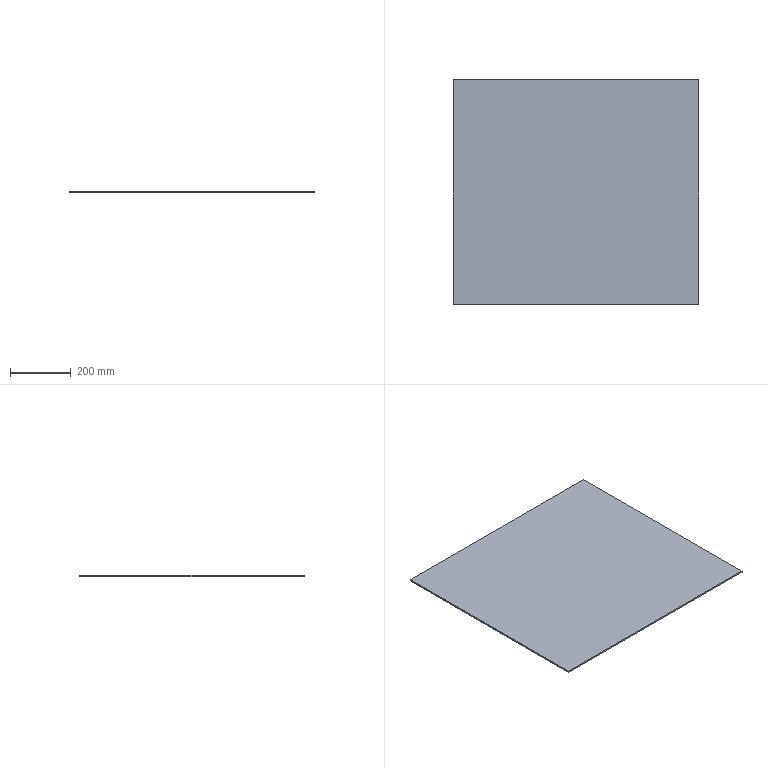Part | STEP file | Guide wheel mechanism revised.sldasm-Part-23 | 1 solid | 6 faces | box 810 x 740 x 5 mm | volume 2997000 mm3 | plane 6
STEP:
#1=CARTESIAN_POINT('',(-405.,740.,-505.));
#2=VERTEX_POINT('',#1);
#3=CARTESIAN_POINT('',(-405.,0.,-505.));
#4=VERTEX_POINT('',#3);
#5=CARTESIAN_POINT('',(-405.,740.,-505.));
#6=DIRECTION('',(0.,-1.,0.));
#7=VECTOR('',#6,1000.);
#8=LINE('',#5,#7);
#9=EDGE_CURVE('',#2,#4,#8,.T.);
#10=ORIENTED_EDGE('',*,*,#9,.F.);
#11=CARTESIAN_POINT('',(-405.,740.,-510.));
#12=VERTEX_POINT('',#11);
#13=CARTESIAN_POINT('',(-405.,740.,-510.));
#14=DIRECTION('',(0.,0.,1.));
#15=VECTOR('',#14,1000.);
#16=LINE('',#13,#15);
#17=EDGE_CURVE('',#12,#2,#16,.T.);
#18=ORIENTED_EDGE('',*,*,#17,.F.);
#19=CARTESIAN_POINT('',(-405.,0.,-510.));
#20=VERTEX_POINT('',#19);
#21=CARTESIAN_POINT('',(-405.,740.,-510.));
#22=DIRECTION('',(0.,-1.,0.));
#23=VECTOR('',#22,1000.);
#24=LINE('',#21,#23);
#25=EDGE_CURVE('',#12,#20,#24,.T.);
#26=ORIENTED_EDGE('',*,*,#25,.T.);
#27=CARTESIAN_POINT('',(-405.,0.,-510.));
#28=DIRECTION('',(0.,0.,1.));
#29=VECTOR('',#28,1000.);
#30=LINE('',#27,#29);
#31=EDGE_CURVE('',#20,#4,#30,.T.);
#32=ORIENTED_EDGE('',*,*,#31,.T.);
#33=EDGE_LOOP('',(#10,#18,#26,#32));
#34=FACE_OUTER_BOUND('',#33,.T.);
#35=CARTESIAN_POINT('',(-405.,740.,-510.));
#36=DIRECTION('',(-1.,0.,0.));
#37=DIRECTION('',(0.,-1.,0.));
#38=AXIS2_PLACEMENT_3D('',#35,#36,#37);
#39=PLANE('',#38);
#40=ADVANCED_FACE('',(#34),#39,.T.);
#41=CARTESIAN_POINT('',(405.,740.,-505.));
#42=VERTEX_POINT('',#41);
#43=CARTESIAN_POINT('',(-405.,740.,-505.));
#44=DIRECTION('',(-1.,0.,0.));
#45=VECTOR('',#44,1000.);
#46=LINE('',#43,#45);
#47=EDGE_CURVE('',#42,#2,#46,.T.);
#48=ORIENTED_EDGE('',*,*,#47,.F.);
#49=CARTESIAN_POINT('',(405.,740.,-510.));
#50=VERTEX_POINT('',#49);
#51=CARTESIAN_POINT('',(405.,740.,-510.));
#52=DIRECTION('',(0.,0.,1.));
#53=VECTOR('',#52,1000.);
#54=LINE('',#51,#53);
#55=EDGE_CURVE('',#50,#42,#54,.T.);
#56=ORIENTED_EDGE('',*,*,#55,.F.);
#57=CARTESIAN_POINT('',(-405.,740.,-510.));
#58=DIRECTION('',(-1.,0.,0.));
#59=VECTOR('',#58,1000.);
#60=LINE('',#57,#59);
#61=EDGE_CURVE('',#50,#12,#60,.T.);
#62=ORIENTED_EDGE('',*,*,#61,.T.);
#63=ORIENTED_EDGE('',*,*,#17,.T.);
#64=EDGE_LOOP('',(#48,#56,#62,#63));
#65=FACE_OUTER_BOUND('',#64,.T.);
#66=CARTESIAN_POINT('',(-405.,740.,-510.));
#67=DIRECTION('',(0.,1.,0.));
#68=DIRECTION('',(0.,0.,1.));
#69=AXIS2_PLACEMENT_3D('',#66,#67,#68);
#70=PLANE('',#69);
#71=ADVANCED_FACE('',(#65),#70,.T.);
#72=CARTESIAN_POINT('',(405.,0.,-505.));
#73=VERTEX_POINT('',#72);
#74=CARTESIAN_POINT('',(405.,740.,-505.));
#75=DIRECTION('',(0.,1.,0.));
#76=VECTOR('',#75,1000.);
#77=LINE('',#74,#76);
#78=EDGE_CURVE('',#73,#42,#77,.T.);
#79=ORIENTED_EDGE('',*,*,#78,.F.);
#80=CARTESIAN_POINT('',(405.,0.,-510.));
#81=VERTEX_POINT('',#80);
#82=CARTESIAN_POINT('',(405.,0.,-510.));
#83=DIRECTION('',(0.,0.,1.));
#84=VECTOR('',#83,1000.);
#85=LINE('',#82,#84);
#86=EDGE_CURVE('',#81,#73,#85,.T.);
#87=ORIENTED_EDGE('',*,*,#86,.F.);
#88=CARTESIAN_POINT('',(405.,740.,-510.));
#89=DIRECTION('',(0.,1.,0.));
#90=VECTOR('',#89,1000.);
#91=LINE('',#88,#90);
#92=EDGE_CURVE('',#81,#50,#91,.T.);
#93=ORIENTED_EDGE('',*,*,#92,.T.);
#94=ORIENTED_EDGE('',*,*,#55,.T.);
#95=EDGE_LOOP('',(#79,#87,#93,#94));
#96=FACE_OUTER_BOUND('',#95,.T.);
#97=CARTESIAN_POINT('',(405.,740.,-510.));
#98=DIRECTION('',(1.,0.,0.));
#99=DIRECTION('',(0.,1.,0.));
#100=AXIS2_PLACEMENT_3D('',#97,#98,#99);
#101=PLANE('',#100);
#102=ADVANCED_FACE('',(#96),#101,.T.);
#103=CARTESIAN_POINT('',(-405.,0.,-505.));
#104=DIRECTION('',(1.,0.,0.));
#105=VECTOR('',#104,1000.);
#106=LINE('',#103,#105);
#107=EDGE_CURVE('',#4,#73,#106,.T.);
#108=ORIENTED_EDGE('',*,*,#107,.F.);
#109=ORIENTED_EDGE('',*,*,#31,.F.);
#110=CARTESIAN_POINT('',(-405.,0.,-510.));
#111=DIRECTION('',(1.,0.,0.));
#112=VECTOR('',#111,1000.);
#113=LINE('',#110,#112);
#114=EDGE_CURVE('',#20,#81,#113,.T.);
#115=ORIENTED_EDGE('',*,*,#114,.T.);
#116=ORIENTED_EDGE('',*,*,#86,.T.);
#117=EDGE_LOOP('',(#108,#109,#115,#116));
#118=FACE_OUTER_BOUND('',#117,.T.);
#119=CARTESIAN_POINT('',(-405.,0.,-510.));
#120=DIRECTION('',(0.,-1.,0.));
#121=DIRECTION('',(0.,0.,-1.));
#122=AXIS2_PLACEMENT_3D('',#119,#120,#121);
#123=PLANE('',#122);
#124=ADVANCED_FACE('',(#118),#123,.T.);
#125=ORIENTED_EDGE('',*,*,#25,.F.);
#126=ORIENTED_EDGE('',*,*,#61,.F.);
#127=ORIENTED_EDGE('',*,*,#92,.F.);
#128=ORIENTED_EDGE('',*,*,#114,.F.);
#129=EDGE_LOOP('',(#125,#126,#127,#128));
#130=FACE_OUTER_BOUND('',#129,.T.);
#131=CARTESIAN_POINT('',(0.,0.,-510.));
#132=DIRECTION('',(0.,0.,1.));
#133=DIRECTION('',(1.,0.,0.));
#134=AXIS2_PLACEMENT_3D('',#131,#132,#133);
#135=PLANE('',#134);
#136=ADVANCED_FACE('',(#130),#135,.F.);
#137=ORIENTED_EDGE('',*,*,#9,.T.);
#138=ORIENTED_EDGE('',*,*,#107,.T.);
#139=ORIENTED_EDGE('',*,*,#78,.T.);
#140=ORIENTED_EDGE('',*,*,#47,.T.);
#141=EDGE_LOOP('',(#137,#138,#139,#140));
#142=FACE_OUTER_BOUND('',#141,.T.);
#143=CARTESIAN_POINT('',(0.,0.,-505.));
#144=DIRECTION('',(0.,0.,1.));
#145=DIRECTION('',(1.,0.,0.));
#146=AXIS2_PLACEMENT_3D('',#143,#144,#145);
#147=PLANE('',#146);
#148=ADVANCED_FACE('',(#142),#147,.T.);
#149=CLOSED_SHELL('',(#40,#71,#102,#124,#136,#148));
#150=MANIFOLD_SOLID_BREP('',#149);
#151=CARTESIAN_POINT('',(0.,0.,0.));
#152=DIRECTION('',(0.,0.,1.));
#153=DIRECTION('',(1.,0.,0.));
#154=AXIS2_PLACEMENT_3D('',#151,#152,#153);
#155=(LENGTH_UNIT()NAMED_UNIT(*)SI_UNIT(.MILLI.,.METRE.));
#156=UNCERTAINTY_MEASURE_WITH_UNIT(LENGTH_MEASURE(0.00001),#155,'','');
#157=(NAMED_UNIT(*)PLANE_ANGLE_UNIT()SI_UNIT($,.RADIAN.));
#158=(NAMED_UNIT(*)SI_UNIT($,.STERADIAN.)SOLID_ANGLE_UNIT());
#159=(GEOMETRIC_REPRESENTATION_CONTEXT(3)GLOBAL_UNCERTAINTY_ASSIGNED_CONTEXT((#156))GLOBAL_UNIT_ASSIGNED_CONTEXT((#155,#157,#158))REPRESENTATION_CONTEXT('',''));
#160=ADVANCED_BREP_SHAPE_REPRESENTATION('',(#150,#154),#159);